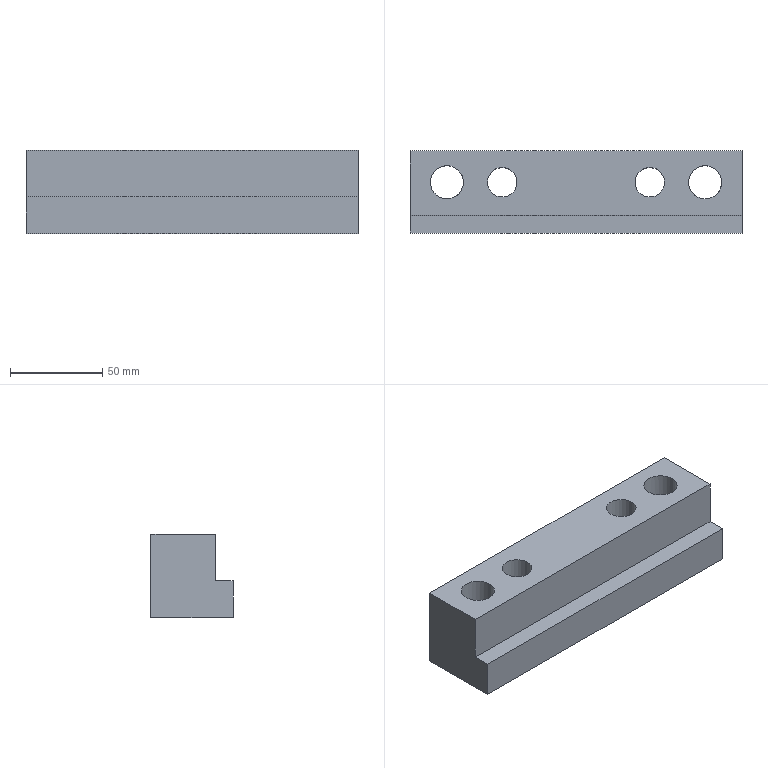Part | STEP file | solid 206 | 1 solid | 16 faces | box 180 x 44.5 x 45 mm | volume 267303 mm3 | plane 10 | cylinder 6 | commonest cylinder face diameters 16 x2 18 x2 26 x2